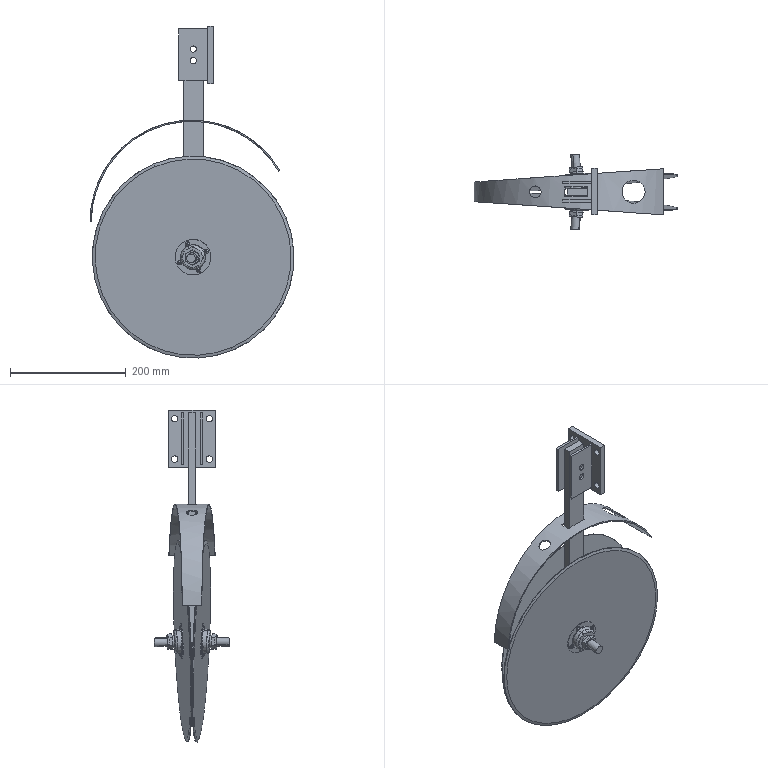Part | SolidWorks | features ReferencePattern 7, CompositeCurve 3, MirrorCompFeat 2 | 20 solids | 373 faces | box 353.001 x 130.927 x 574.882 mm | volume 819203 mm3 | cylinder 149 | plane 120 | cone 36 | torus 36 | sphere 32 | commonest cylinder face diameters 4 x48 11 x20 31 x12 19 x9 15 x8 22.27 x8